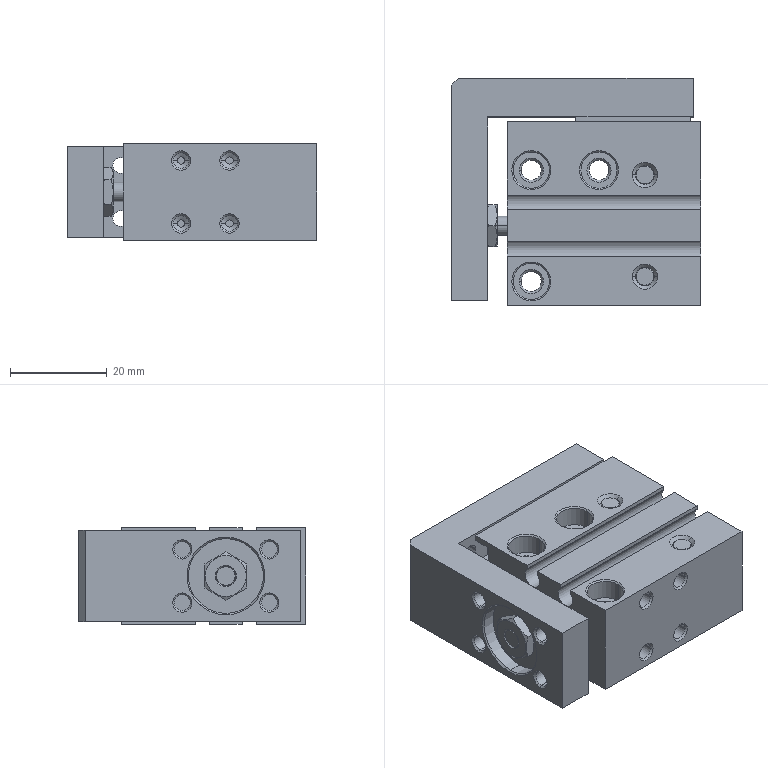Part | STEP file | 2 solids | 358 faces | box 51.5 x 47 x 20 mm | volume 36061 mm3 | cone 130 | cylinder 110 | plane 110 | torus 8 | commonest cylinder face diameters 3.242 x32 4.2 x14 7.5 x12 4.134 x10 0.4 x8 1.74 x8